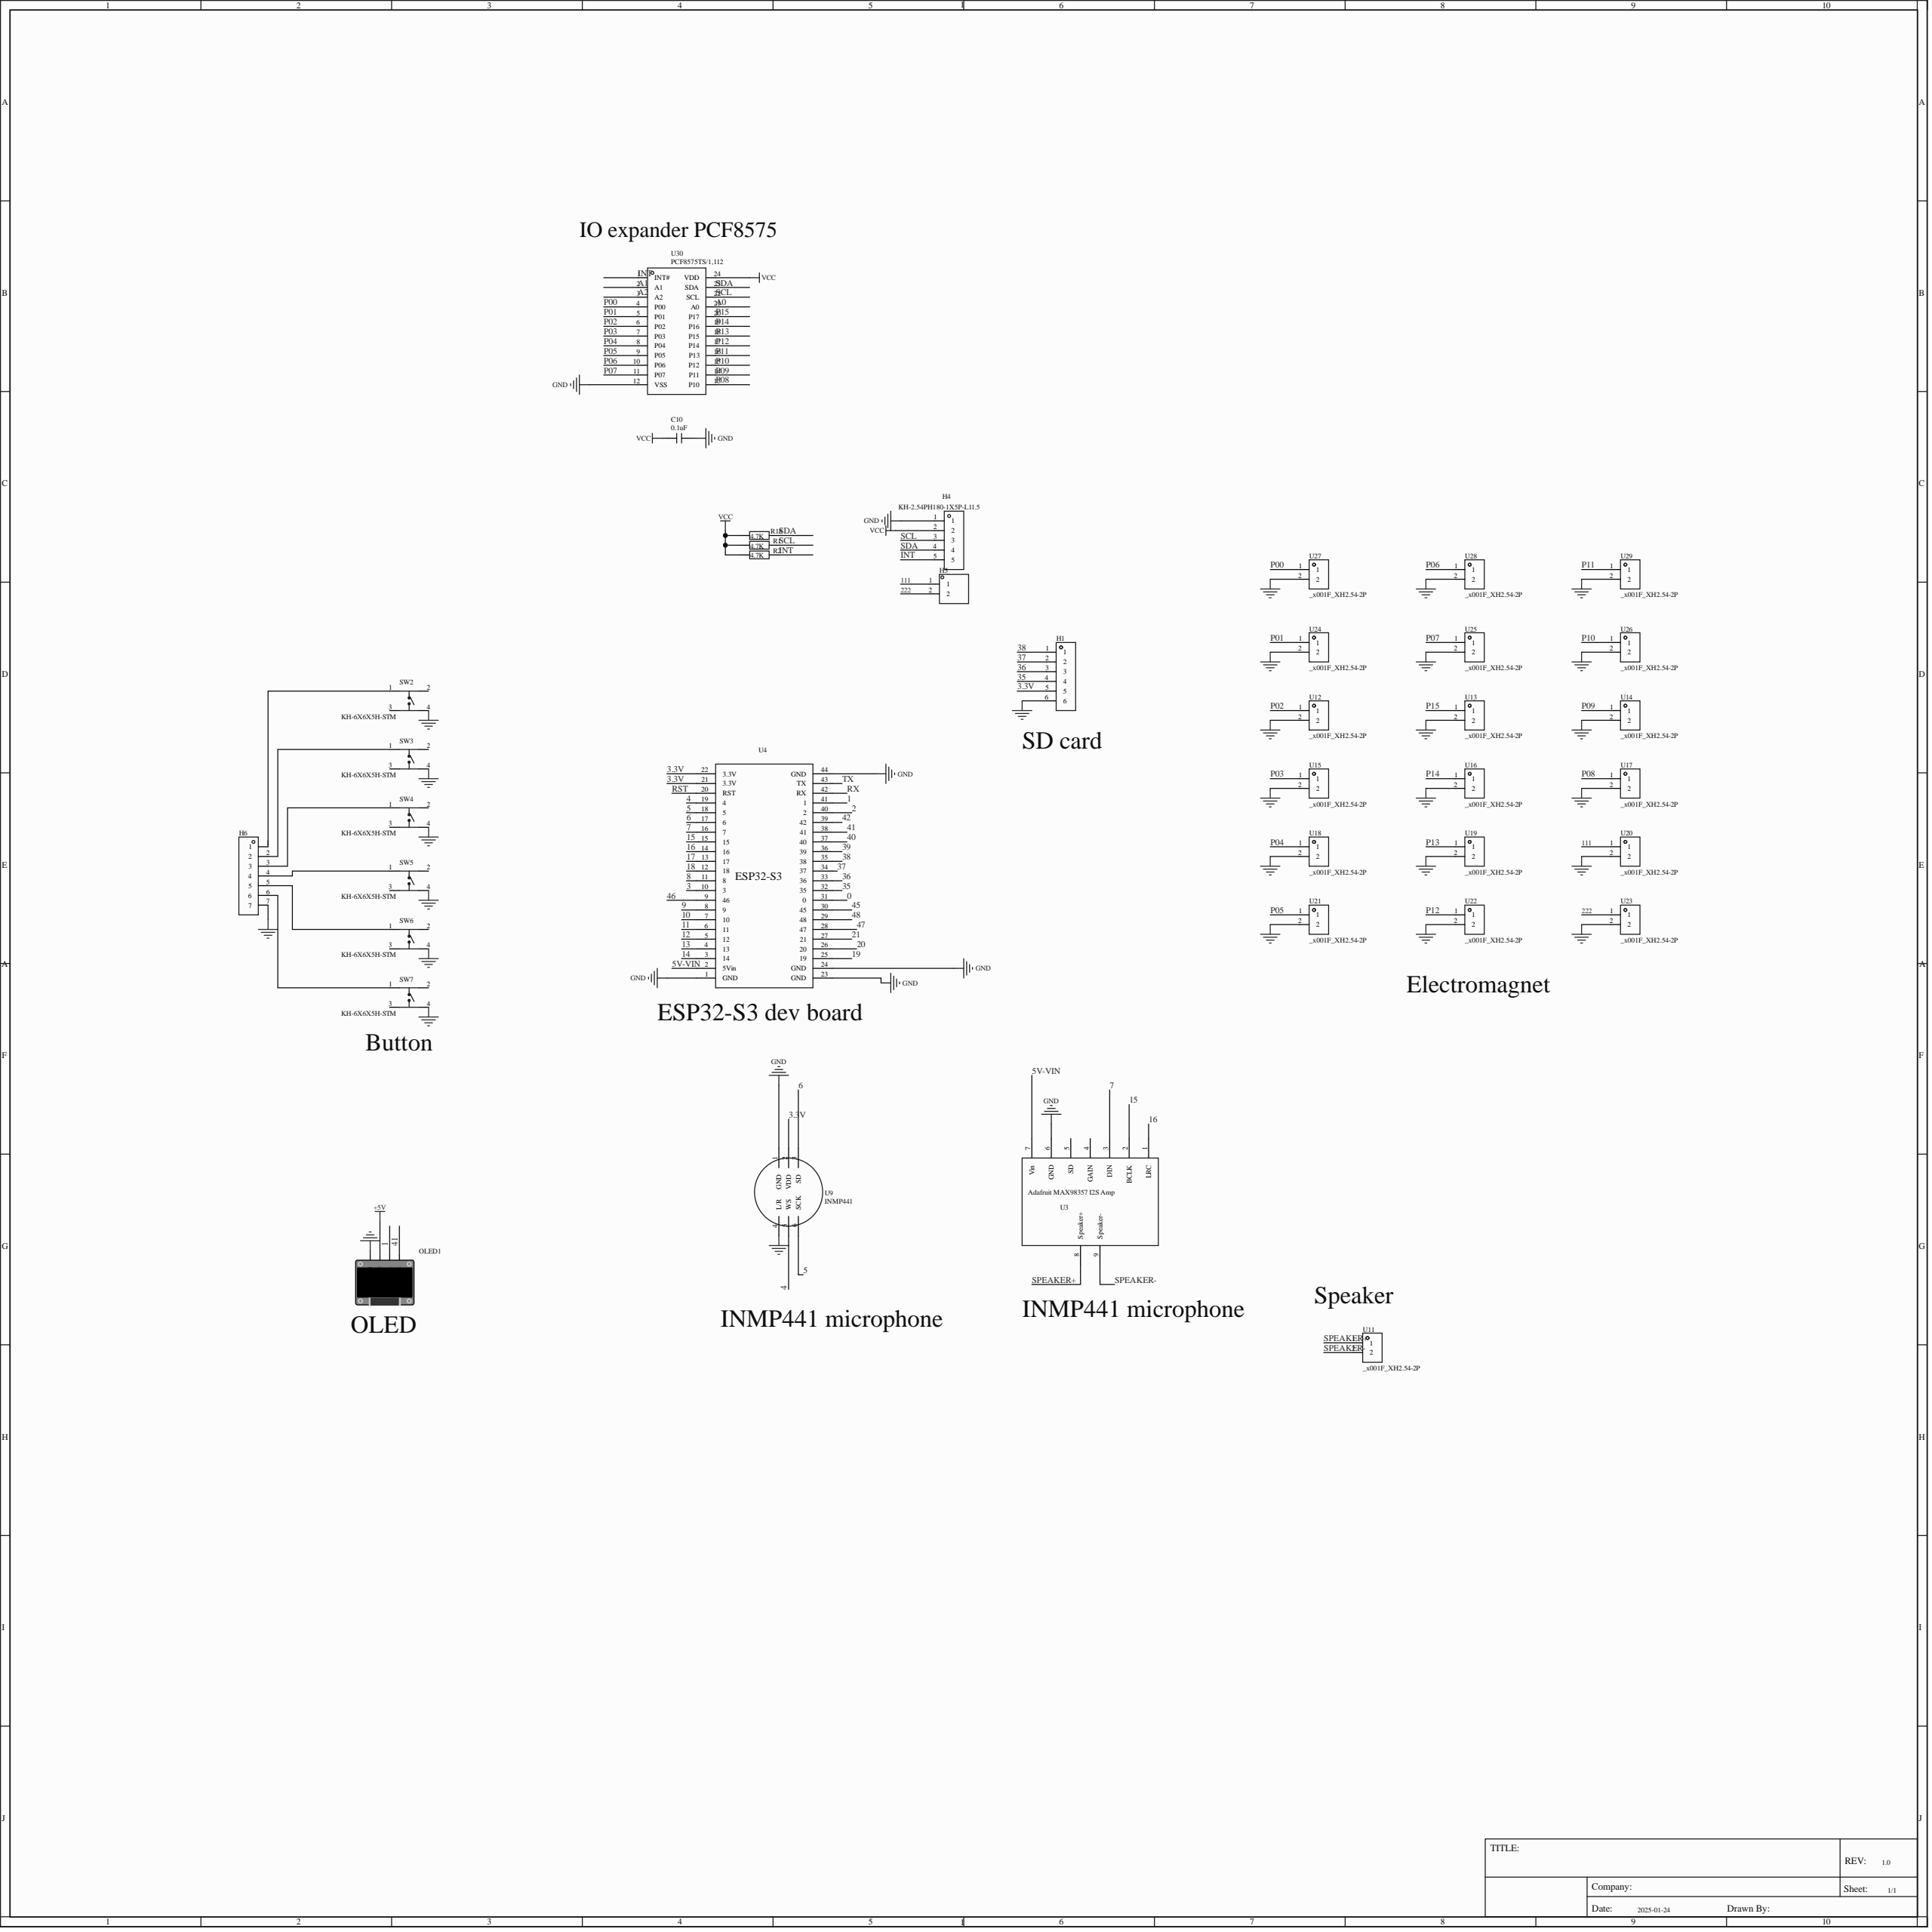Circuit board | Altium Designer | 38 parts | 45 nets
Bill of materials:
Comment,Description,Designator,Footprint,LibRef,Quantity
"0.1uF","","C10","C0603-1","0.1uF","1"
"","","H1","HDR-TH_6P-P2.54-V-F","HDR-F_2.54_1x6P","1"
"KH-2.54PH180-1X5P-L11.5","","H4","HDR-TH_5P-P2.54-V-M","KH-2.54PH180-1X5P-L11.5","1"
"","","H5","HDR-TH_2P-P2.54-V-M-1","HDR-M_2.54_1x2P","1"
"","","H6","HDR-TH_7P-P2.54-V-M","HDR-M_2.54_1x7P","1"
"","","OLED1","0.96OLED_4P","0.96OLED模块_4P","1"
"4.7K","","R1, R2, R18","R0603-1","4.7K","3"
"KH-6X6X5H-STM","Structure: SPST; Actuator: round button; Mounting: upright SMD; Length: 6mm; Width: 6mm; Height: 5mm; With bracket: no; Contact current: 50mA; Rated voltage (DC): 12V; Mechanical life: 8 ten-thousand cycles;","SW2, SW3, SW4, SW5, SW6, SW7","SW-SMD_4P-L6.0-W6.0-P4.50-LS9.0-2","KH-6X6X5H-STM","6"
"Adafruit MAX98357 I2S Amp","","U3","MAX98357 I2S AMP MODULE","Adafruit MAX98357 I2S Amp","1"
"NO","","U4","ESP32S3","NO","1"
"INMP441","","U9","INMP441","INMP441","1"
"_x001F_XH2.54-2P","","U11, U12, U13, U14, U15, U16, U17, U18, U19, U20, U21, U22, U23, U24, U25, U26, U27, U28, U29","CONN-TH_2P-P2.54-V","_x001F_XH2.54-2P","19"
"PCF8575TS/1,112","","U30","SSOP-24_L8.2-W5.3-P0.65-LS7.8-BL","PCF8575TS/1,112","1"
Netlist (Protel format):
[
C10
C0603-1
0.1uF



]
[
H1
HDR-TH_6P-P2.54-V-F




]
[
H4
HDR-TH_5P-P2.54-V-M
KH-2.54PH180-1X5P-L11.5



]
[
H5
HDR-TH_2P-P2.54-V-M-1




]
[
H6
HDR-TH_7P-P2.54-V-M




]
[
OLED1
0.96OLED_4P




]
[
R1
R0603-1
4.7K



]
[
R2
R0603-1
4.7K



]
[
R18
R0603-1
4.7K



]
[
SW2
SW-SMD_4P-L6.0-W6.0-P4.50-LS9.0-2
KH-6X6X5H-STM



]
[
SW3
SW-SMD_4P-L6.0-W6.0-P4.50-LS9.0-2
KH-6X6X5H-STM



]
[
SW4
SW-SMD_4P-L6.0-W6.0-P4.50-LS9.0-2
KH-6X6X5H-STM



]
[
SW5
SW-SMD_4P-L6.0-W6.0-P4.50-LS9.0-2
KH-6X6X5H-STM



]
[
SW6
SW-SMD_4P-L6.0-W6.0-P4.50-LS9.0-2
KH-6X6X5H-STM



]
[
SW7
SW-SMD_4P-L6.0-W6.0-P4.50-LS9.0-2
KH-6X6X5H-STM



]
[
U3
MAX98357 I2S AMP MODULE
Adafruit MAX98357 I2S Amp



]
[
U4
ESP32S3
NO



]
[
U9
INMP441
INMP441



]
[
U11
CONN-TH_2P-P2.54-V
_x001F_XH2.54-2P



]
[
U12
CONN-TH_2P-P2.54-V
_x001F_XH2.54-2P



]
[
U13
CONN-TH_2P-P2.54-V
_x001F_XH2.54-2P



]
[
U14
CONN-TH_2P-P2.54-V
_x001F_XH2.54-2P



]
[
U15
CONN-TH_2P-P2.54-V
_x001F_XH2.54-2P



]
[
U16
CONN-TH_2P-P2.54-V
_x001F_XH2.54-2P



]
[
U17
CONN-TH_2P-P2.54-V
_x001F_XH2.54-2P



]
[
U18
CONN-TH_2P-P2.54-V
_x001F_XH2.54-2P



]
[
U19
CONN-TH_2P-P2.54-V
_x001F_XH2.54-2P



]
[
U20
CONN-TH_2P-P2.54-V
_x001F_XH2.54-2P



]
[
U21
CONN-TH_2P-P2.54-V
_x001F_XH2.54-2P



]
[
U22
CONN-TH_2P-P2.54-V
_x001F_XH2.54-2P



]
[
U23
CONN-TH_2P-P2.54-V
_x001F_XH2.54-2P



]
[
U24
CONN-TH_2P-P2.54-V
_x001F_XH2.54-2P



]
[
U25
CONN-TH_2P-P2.54-V
_x001F_XH2.54-2P



]
[
U26
CONN-TH_2P-P2.54-V
_x001F_XH2.54-2P



]
[
U27
CONN-TH_2P-P2.54-V
_x001F_XH2.54-2P



]
[
U28
CONN-TH_2P-P2.54-V
_x001F_XH2.54-2P



]
[
U29
CONN-TH_2P-P2.54-V
_x001F_XH2.54-2P



]
[
U30
SSOP-24_L8.2-W5.3-P0.65-LS7.8-BL
PCF8575TS/1,112



]
(
VCC
C10-2
H4-2
R1-2
R2-2
R18-2
U30-24
)
(
SPEAKER-
U3-9
U11-2
)
(
SPEAKER+
U3-8
U11-1
)
(
SDA
H4-4
R18-1
U30-23
)
(
SCL
H4-3
R1-1
U30-22
)
(
P15
U13-1
U30-20
)
(
P14
U16-1
U30-19
)
(
P13
U19-1
U30-18
)
(
P12
U22-1
U30-17
)
(
P11
U29-1
U30-16
)
(
P10
U26-1
U30-15
)
(
P09
U14-1
U30-14
)
(
P08
U17-1
U30-13
)
(
P07
U25-1
U30-11
)
(
P06
U28-1
U30-10
)
(
P05
U21-1
U30-9
)
(
P04
U18-1
U30-8
)
(
P03
U15-1
U30-7
)
(
P02
U12-1
U30-6
)
(
P01
U24-1
U30-5
)
(
P00
U27-1
U30-4
)
(
NetH6_6
H6-6
SW7-1
)
(
NetH6_5
H6-5
SW6-1
)
(
NetH6_4
H6-4
SW5-1
)
(
NetH6_3
H6-3
SW4-1
)
(
NetH6_2
H6-2
SW3-1
)
(
NetH6_1
H6-1
SW2-1
)
(
INT
H4-5
R2-1
U30-1
)
(
GND
C10-1
H1-6
H4-1
H6-7
OLED1-1
SW2-4
SW3-4
SW4-4
SW5-4
SW6-4
SW7-4
U3-6
U4-1
U4-23
U4-24
U4-44
U9-1
U9-4
U12-2
U13-2
U14-2
U15-2
U16-2
U17-2
U18-2
U19-2
U20-2
U21-2
U22-2
U23-2
U24-2
U25-2
U26-2
U27-2
U28-2
U29-2
U30-12
)
(
222
H5-2
U23-1
)
(
111
H5-1
U20-1
)
(
41
OLED1-4
U4-38
)
(
38
H1-1
U4-35
)
(
37
H1-2
U4-34
)
(
36
H1-3
U4-33
)
(
35
H1-4
U4-32
)
(
16
U3-1
U4-14
)
(
15
U3-2
U4-15
)
(
7
U3-3
U4-16
)
(
6
U4-17
U9-3
)
(
5V-VIN
U3-7
U4-2
)
(
5
U4-18
U9-6
)
(
4
U4-19
U9-5
)
(
3.3V
H1-5
U4-21
U4-22
U9-2
)
(
1
OLED1-3
U4-41
)